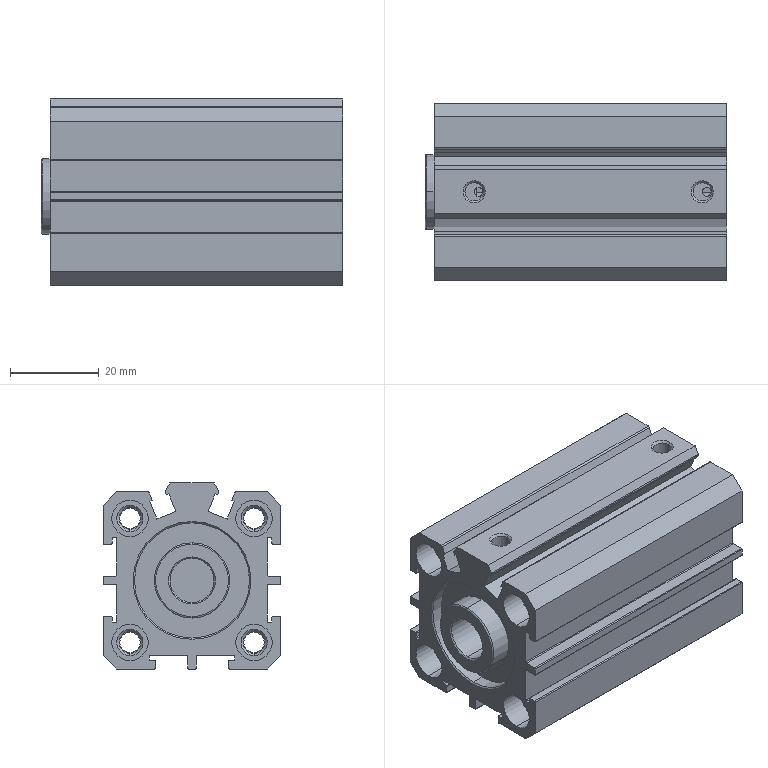Part | SolidWorks | S-SDA25x35-SB_body.stp | 1 solid | 218 faces | box 68 x 40 x 42 mm | volume 59012 mm3 | cylinder 99 | plane 87 | cone 30 | torus 2 | commonest cylinder face diameters 0.4 x36 4.917 x16 8.2 x16 4.6 x8 0.8 x4 2 x4